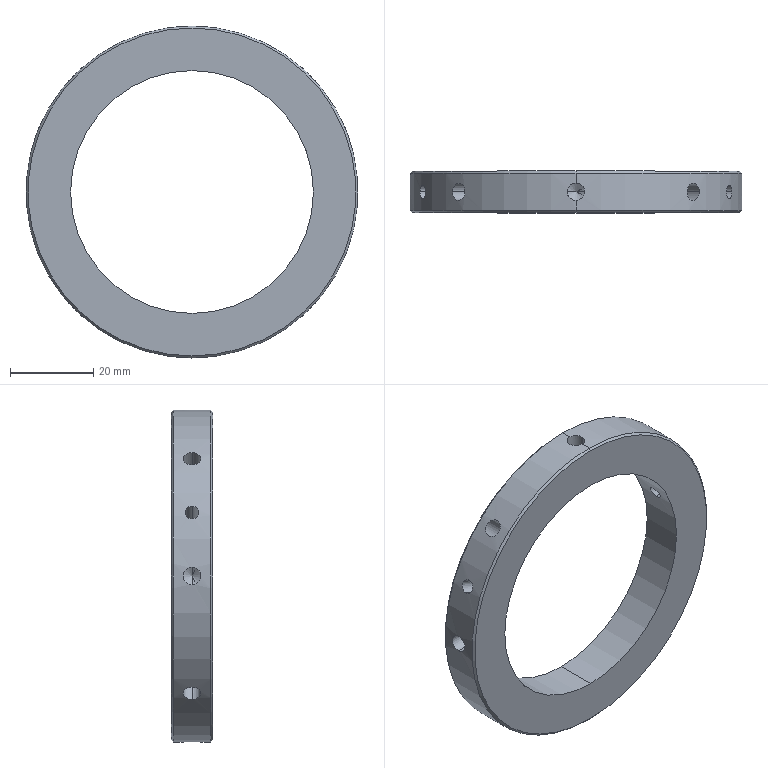Part | SolidWorks | features CirPattern 2, HoleWzd 2, Chamfer 1, Extrusion 1 | 1 solid | 46 faces | box 80 x 10 x 80 mm | volume 22320 mm3 | cylinder 24 | cone 20 | plane 2 | commonest cylinder face diameters 4.2 x16 3.3 x4 58.5 x2 80 x2